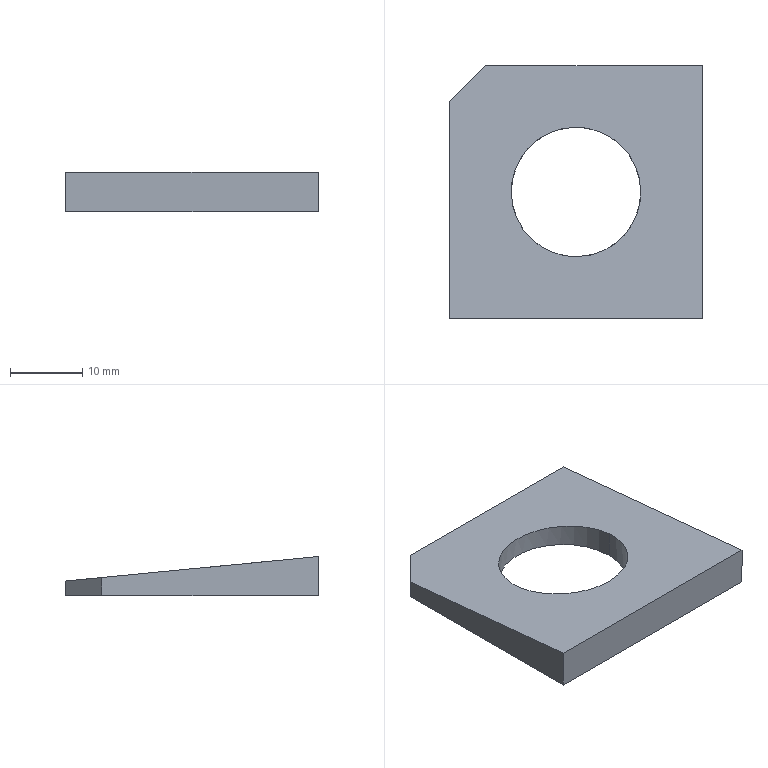Part | SolidWorks | features Cut 2, Extrusion 1 | 1 solid | 9 faces | box 35 x 35 x 5.4 mm | volume 3571 mm3 | plane 7 | cylinder 2 | commonest cylinder face diameters 17.93 x2
STEP:
#1=CARTESIAN_POINT('',(-8.965,0.,3.7));
#2=VERTEX_POINT('',#1);
#3=CARTESIAN_POINT('',(8.965,0.,3.7));
#4=VERTEX_POINT('',#3);
#5=CARTESIAN_POINT('',(-8.965,0.,3.7));
#6=CARTESIAN_POINT('',(-8.965,-17.93,5.442));
#7=CARTESIAN_POINT('',(8.965,-17.93,5.442));
#8=CARTESIAN_POINT('',(8.965,0.,3.7));
#9=(BOUNDED_CURVE()B_SPLINE_CURVE(3,(#5,#6,#7,#8),.UNSPECIFIED.,.F.,.F.)B_SPLINE_CURVE_WITH_KNOTS((4,4),(1.571,4.712),.UNSPECIFIED.)CURVE()GEOMETRIC_REPRESENTATION_ITEM()RATIONAL_B_SPLINE_CURVE((1.,0.3333,0.3333,1.))REPRESENTATION_ITEM(''));
#10=EDGE_CURVE('',#2,#4,#9,.T.);
#11=ORIENTED_EDGE('',*,*,#10,.T.);
#12=CARTESIAN_POINT('',(8.965,0.,0.));
#13=VERTEX_POINT('',#12);
#14=CARTESIAN_POINT('',(8.965,0.,5.4));
#15=DIRECTION('',(0.,0.,-1.));
#16=VECTOR('',#15,1000.);
#17=LINE('',#14,#16);
#18=EDGE_CURVE('',#4,#13,#17,.T.);
#19=ORIENTED_EDGE('',*,*,#18,.T.);
#20=CARTESIAN_POINT('',(-8.965,0.,0.));
#21=VERTEX_POINT('',#20);
#22=CARTESIAN_POINT('',(0.,0.,0.));
#23=DIRECTION('',(0.,0.,1.));
#24=DIRECTION('',(1.,0.,0.));
#25=AXIS2_PLACEMENT_3D('',#22,#23,#24);
#26=CIRCLE('',#25,8.965);
#27=EDGE_CURVE('',#21,#13,#26,.T.);
#28=ORIENTED_EDGE('',*,*,#27,.F.);
#29=CARTESIAN_POINT('',(-8.965,0.,5.4));
#30=DIRECTION('',(0.,0.,-1.));
#31=VECTOR('',#30,1000.);
#32=LINE('',#29,#31);
#33=EDGE_CURVE('',#2,#21,#32,.T.);
#34=ORIENTED_EDGE('',*,*,#33,.F.);
#35=EDGE_LOOP('',(#11,#19,#28,#34));
#36=FACE_OUTER_BOUND('',#35,.T.);
#37=CARTESIAN_POINT('',(0.,0.,5.4));
#38=DIRECTION('',(0.,0.,-1.));
#39=DIRECTION('',(-1.,0.,0.));
#40=AXIS2_PLACEMENT_3D('',#37,#38,#39);
#41=CYLINDRICAL_SURFACE('',#40,8.965);
#42=ADVANCED_FACE('',(#36),#41,.F.);
#43=CARTESIAN_POINT('',(-17.5,-17.5,5.4));
#44=VERTEX_POINT('',#43);
#45=CARTESIAN_POINT('',(-17.5,12.5,2.486));
#46=VERTEX_POINT('',#45);
#47=CARTESIAN_POINT('',(-17.5,-17.5,5.4));
#48=DIRECTION('',(0.,0.9953,-0.09669));
#49=VECTOR('',#48,1000.);
#50=LINE('',#47,#49);
#51=EDGE_CURVE('',#44,#46,#50,.T.);
#52=ORIENTED_EDGE('',*,*,#51,.T.);
#53=CARTESIAN_POINT('',(-17.5,12.5,0.));
#54=VERTEX_POINT('',#53);
#55=CARTESIAN_POINT('',(-17.5,12.5,5.4));
#56=DIRECTION('',(0.,0.,-1.));
#57=VECTOR('',#56,1000.);
#58=LINE('',#55,#57);
#59=EDGE_CURVE('',#46,#54,#58,.T.);
#60=ORIENTED_EDGE('',*,*,#59,.T.);
#61=CARTESIAN_POINT('',(-17.5,-17.5,0.));
#62=VERTEX_POINT('',#61);
#63=CARTESIAN_POINT('',(-17.5,17.5,0.));
#64=DIRECTION('',(0.,-1.,0.));
#65=VECTOR('',#64,1000.);
#66=LINE('',#63,#65);
#67=EDGE_CURVE('',#54,#62,#66,.T.);
#68=ORIENTED_EDGE('',*,*,#67,.T.);
#69=CARTESIAN_POINT('',(-17.5,-17.5,5.4));
#70=DIRECTION('',(0.,0.,-1.));
#71=VECTOR('',#70,1000.);
#72=LINE('',#69,#71);
#73=EDGE_CURVE('',#44,#62,#72,.T.);
#74=ORIENTED_EDGE('',*,*,#73,.F.);
#75=EDGE_LOOP('',(#52,#60,#68,#74));
#76=FACE_OUTER_BOUND('',#75,.T.);
#77=CARTESIAN_POINT('',(-17.5,17.5,5.4));
#78=DIRECTION('',(1.,0.,0.));
#79=DIRECTION('',(0.,0.,-1.));
#80=AXIS2_PLACEMENT_3D('',#77,#78,#79);
#81=PLANE('',#80);
#82=ADVANCED_FACE('',(#76),#81,.F.);
#83=CARTESIAN_POINT('',(17.5,17.5,2.));
#84=VERTEX_POINT('',#83);
#85=CARTESIAN_POINT('',(17.5,-17.5,5.4));
#86=VERTEX_POINT('',#85);
#87=CARTESIAN_POINT('',(17.5,-17.5,5.4));
#88=DIRECTION('',(0.,-0.9953,0.09669));
#89=VECTOR('',#88,1000.);
#90=LINE('',#87,#89);
#91=EDGE_CURVE('',#84,#86,#90,.T.);
#92=ORIENTED_EDGE('',*,*,#91,.T.);
#93=CARTESIAN_POINT('',(17.5,-17.5,0.));
#94=VERTEX_POINT('',#93);
#95=CARTESIAN_POINT('',(17.5,-17.5,5.4));
#96=DIRECTION('',(0.,0.,-1.));
#97=VECTOR('',#96,1000.);
#98=LINE('',#95,#97);
#99=EDGE_CURVE('',#86,#94,#98,.T.);
#100=ORIENTED_EDGE('',*,*,#99,.T.);
#101=CARTESIAN_POINT('',(17.5,17.5,0.));
#102=VERTEX_POINT('',#101);
#103=CARTESIAN_POINT('',(17.5,17.5,0.));
#104=DIRECTION('',(0.,1.,0.));
#105=VECTOR('',#104,1000.);
#106=LINE('',#103,#105);
#107=EDGE_CURVE('',#94,#102,#106,.T.);
#108=ORIENTED_EDGE('',*,*,#107,.T.);
#109=CARTESIAN_POINT('',(17.5,17.5,5.4));
#110=DIRECTION('',(0.,0.,-1.));
#111=VECTOR('',#110,1000.);
#112=LINE('',#109,#111);
#113=EDGE_CURVE('',#84,#102,#112,.T.);
#114=ORIENTED_EDGE('',*,*,#113,.F.);
#115=EDGE_LOOP('',(#92,#100,#108,#114));
#116=FACE_OUTER_BOUND('',#115,.T.);
#117=CARTESIAN_POINT('',(17.5,17.5,5.4));
#118=DIRECTION('',(-1.,0.,0.));
#119=DIRECTION('',(0.,-1.,0.));
#120=AXIS2_PLACEMENT_3D('',#117,#118,#119);
#121=PLANE('',#120);
#122=ADVANCED_FACE('',(#116),#121,.F.);
#123=CARTESIAN_POINT('',(-12.5,17.5,0.));
#124=VERTEX_POINT('',#123);
#125=CARTESIAN_POINT('',(-17.5,17.5,0.));
#126=DIRECTION('',(-1.,0.,0.));
#127=VECTOR('',#126,1000.);
#128=LINE('',#125,#127);
#129=EDGE_CURVE('',#102,#124,#128,.T.);
#130=ORIENTED_EDGE('',*,*,#129,.T.);
#131=CARTESIAN_POINT('',(-12.5,17.5,2.));
#132=VERTEX_POINT('',#131);
#133=CARTESIAN_POINT('',(-12.5,17.5,5.4));
#134=DIRECTION('',(0.,0.,-1.));
#135=VECTOR('',#134,1000.);
#136=LINE('',#133,#135);
#137=EDGE_CURVE('',#132,#124,#136,.T.);
#138=ORIENTED_EDGE('',*,*,#137,.F.);
#139=CARTESIAN_POINT('',(-53.268,17.5,2.));
#140=DIRECTION('',(1.,0.,0.));
#141=VECTOR('',#140,1000.);
#142=LINE('',#139,#141);
#143=EDGE_CURVE('',#132,#84,#142,.T.);
#144=ORIENTED_EDGE('',*,*,#143,.T.);
#145=ORIENTED_EDGE('',*,*,#113,.T.);
#146=EDGE_LOOP('',(#130,#138,#144,#145));
#147=FACE_OUTER_BOUND('',#146,.T.);
#148=CARTESIAN_POINT('',(-17.5,17.5,5.4));
#149=DIRECTION('',(0.,-1.,0.));
#150=DIRECTION('',(1.,0.,0.));
#151=AXIS2_PLACEMENT_3D('',#148,#149,#150);
#152=PLANE('',#151);
#153=ADVANCED_FACE('',(#147),#152,.F.);
#154=ORIENTED_EDGE('',*,*,#18,.F.);
#155=CARTESIAN_POINT('',(8.965,0.,3.7));
#156=CARTESIAN_POINT('',(8.965,17.93,1.958));
#157=CARTESIAN_POINT('',(-8.965,17.93,1.958));
#158=CARTESIAN_POINT('',(-8.965,0.,3.7));
#159=(BOUNDED_CURVE()B_SPLINE_CURVE(3,(#155,#156,#157,#158),.UNSPECIFIED.,.F.,.F.)B_SPLINE_CURVE_WITH_KNOTS((4,4),(4.712,7.854),.UNSPECIFIED.)CURVE()GEOMETRIC_REPRESENTATION_ITEM()RATIONAL_B_SPLINE_CURVE((1.,0.3333,0.3333,1.))REPRESENTATION_ITEM(''));
#160=EDGE_CURVE('',#4,#2,#159,.T.);
#161=ORIENTED_EDGE('',*,*,#160,.T.);
#162=ORIENTED_EDGE('',*,*,#33,.T.);
#163=CARTESIAN_POINT('',(0.,0.,0.));
#164=DIRECTION('',(0.,0.,1.));
#165=DIRECTION('',(1.,0.,0.));
#166=AXIS2_PLACEMENT_3D('',#163,#164,#165);
#167=CIRCLE('',#166,8.965);
#168=EDGE_CURVE('',#13,#21,#167,.T.);
#169=ORIENTED_EDGE('',*,*,#168,.F.);
#170=EDGE_LOOP('',(#154,#161,#162,#169));
#171=FACE_OUTER_BOUND('',#170,.T.);
#172=CARTESIAN_POINT('',(0.,0.,5.4));
#173=DIRECTION('',(0.,0.,-1.));
#174=DIRECTION('',(-1.,0.,0.));
#175=AXIS2_PLACEMENT_3D('',#172,#173,#174);
#176=CYLINDRICAL_SURFACE('',#175,8.965);
#177=ADVANCED_FACE('',(#171),#176,.F.);
#178=ORIENTED_EDGE('',*,*,#67,.F.);
#179=CARTESIAN_POINT('',(-12.5,17.5,0.));
#180=DIRECTION('',(-0.7071,-0.7071,0.));
#181=VECTOR('',#180,1000.);
#182=LINE('',#179,#181);
#183=EDGE_CURVE('',#124,#54,#182,.T.);
#184=ORIENTED_EDGE('',*,*,#183,.F.);
#185=ORIENTED_EDGE('',*,*,#129,.F.);
#186=ORIENTED_EDGE('',*,*,#107,.F.);
#187=CARTESIAN_POINT('',(-17.5,-17.5,0.));
#188=DIRECTION('',(1.,0.,0.));
#189=VECTOR('',#188,1000.);
#190=LINE('',#187,#189);
#191=EDGE_CURVE('',#62,#94,#190,.T.);
#192=ORIENTED_EDGE('',*,*,#191,.F.);
#193=EDGE_LOOP('',(#178,#184,#185,#186,#192));
#194=FACE_OUTER_BOUND('',#193,.T.);
#195=ORIENTED_EDGE('',*,*,#27,.T.);
#196=ORIENTED_EDGE('',*,*,#168,.T.);
#197=EDGE_LOOP('',(#195,#196));
#198=FACE_BOUND('',#197,.T.);
#199=CARTESIAN_POINT('',(-17.5,17.5,0.));
#200=DIRECTION('',(0.,0.,1.));
#201=DIRECTION('',(1.,0.,0.));
#202=AXIS2_PLACEMENT_3D('',#199,#200,#201);
#203=PLANE('',#202);
#204=ADVANCED_FACE('',(#194,#198),#203,.F.);
#205=ORIENTED_EDGE('',*,*,#191,.T.);
#206=ORIENTED_EDGE('',*,*,#99,.F.);
#207=CARTESIAN_POINT('',(-17.5,-17.5,5.4));
#208=DIRECTION('',(1.,0.,0.));
#209=VECTOR('',#208,1000.);
#210=LINE('',#207,#209);
#211=EDGE_CURVE('',#44,#86,#210,.T.);
#212=ORIENTED_EDGE('',*,*,#211,.F.);
#213=ORIENTED_EDGE('',*,*,#73,.T.);
#214=EDGE_LOOP('',(#205,#206,#212,#213));
#215=FACE_OUTER_BOUND('',#214,.T.);
#216=CARTESIAN_POINT('',(-17.5,-17.5,5.4));
#217=DIRECTION('',(0.,1.,0.));
#218=DIRECTION('',(-1.,0.,0.));
#219=AXIS2_PLACEMENT_3D('',#216,#217,#218);
#220=PLANE('',#219);
#221=ADVANCED_FACE('',(#215),#220,.F.);
#222=CARTESIAN_POINT('',(-50.371,-20.371,5.679));
#223=DIRECTION('',(0.7054,0.7054,-0.06853));
#224=VECTOR('',#223,1000.);
#225=LINE('',#222,#224);
#226=EDGE_CURVE('',#46,#132,#225,.T.);
#227=ORIENTED_EDGE('',*,*,#226,.F.);
#228=ORIENTED_EDGE('',*,*,#51,.F.);
#229=ORIENTED_EDGE('',*,*,#211,.T.);
#230=ORIENTED_EDGE('',*,*,#91,.F.);
#231=ORIENTED_EDGE('',*,*,#143,.F.);
#232=EDGE_LOOP('',(#227,#228,#229,#230,#231));
#233=FACE_OUTER_BOUND('',#232,.T.);
#234=ORIENTED_EDGE('',*,*,#10,.F.);
#235=ORIENTED_EDGE('',*,*,#160,.F.);
#236=EDGE_LOOP('',(#234,#235));
#237=FACE_BOUND('',#236,.T.);
#238=CARTESIAN_POINT('',(-53.268,-17.5,5.4));
#239=DIRECTION('',(0.,0.09669,0.9953));
#240=DIRECTION('',(0.,-0.9953,0.09669));
#241=AXIS2_PLACEMENT_3D('',#238,#239,#240);
#242=PLANE('',#241);
#243=ADVANCED_FACE('',(#233,#237),#242,.T.);
#244=ORIENTED_EDGE('',*,*,#226,.T.);
#245=ORIENTED_EDGE('',*,*,#137,.T.);
#246=ORIENTED_EDGE('',*,*,#183,.T.);
#247=ORIENTED_EDGE('',*,*,#59,.F.);
#248=EDGE_LOOP('',(#244,#245,#246,#247));
#249=FACE_OUTER_BOUND('',#248,.T.);
#250=CARTESIAN_POINT('',(-12.5,17.5,5.4));
#251=DIRECTION('',(0.7071,-0.7071,0.));
#252=DIRECTION('',(0.7071,0.7071,0.));
#253=AXIS2_PLACEMENT_3D('',#250,#251,#252);
#254=PLANE('',#253);
#255=ADVANCED_FACE('',(#249),#254,.F.);
#256=CLOSED_SHELL('',(#42,#82,#122,#153,#177,#204,#221,#243,#255));
#257=MANIFOLD_SOLID_BREP('',#256);
#258=CARTESIAN_POINT('',(0.,0.,0.));
#259=DIRECTION('',(0.,0.,1.));
#260=DIRECTION('',(1.,0.,0.));
#261=AXIS2_PLACEMENT_3D('',#258,#259,#260);
#262=(LENGTH_UNIT()NAMED_UNIT(*)SI_UNIT(.MILLI.,.METRE.));
#263=UNCERTAINTY_MEASURE_WITH_UNIT(LENGTH_MEASURE(0.00001),#262,'','');
#264=(NAMED_UNIT(*)PLANE_ANGLE_UNIT()SI_UNIT($,.RADIAN.));
#265=(NAMED_UNIT(*)SI_UNIT($,.STERADIAN.)SOLID_ANGLE_UNIT());
#266=(GEOMETRIC_REPRESENTATION_CONTEXT(3)GLOBAL_UNCERTAINTY_ASSIGNED_CONTEXT((#263))GLOBAL_UNIT_ASSIGNED_CONTEXT((#262,#264,#265))REPRESENTATION_CONTEXT('',''));
#267=ADVANCED_BREP_SHAPE_REPRESENTATION('',(#257,#261),#266);